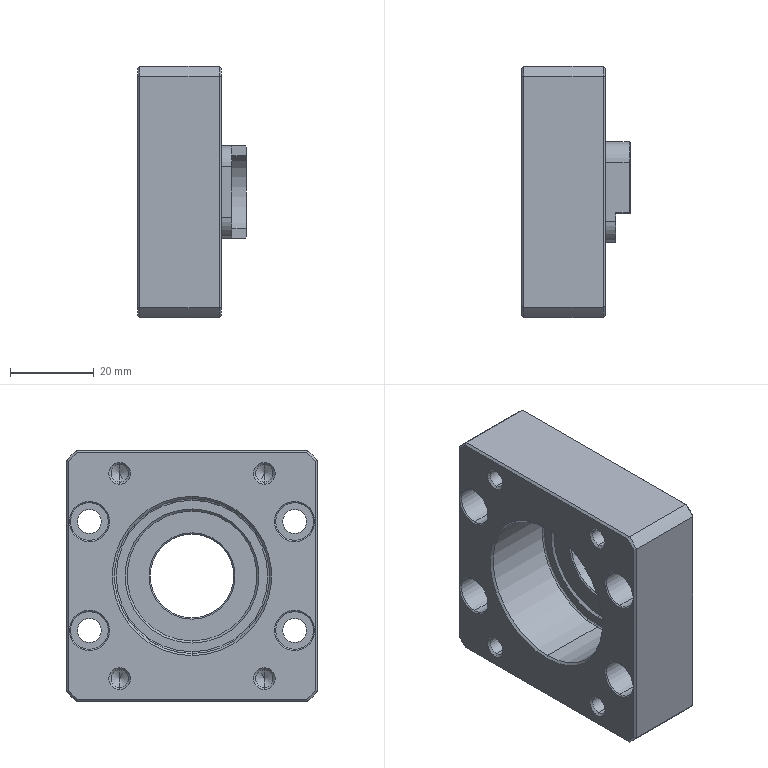Part | SolidWorks | features BaseBody 1 | 1 solid | 117 faces | box 26 x 60 x 60 mm | volume 48842 mm3 | cone 48 | cylinder 36 | plane 31 | torus 2 | commonest cylinder face diameters 4.2 x8 5.7 x8 9 x8 10 x4 81.5 x4 20 x2